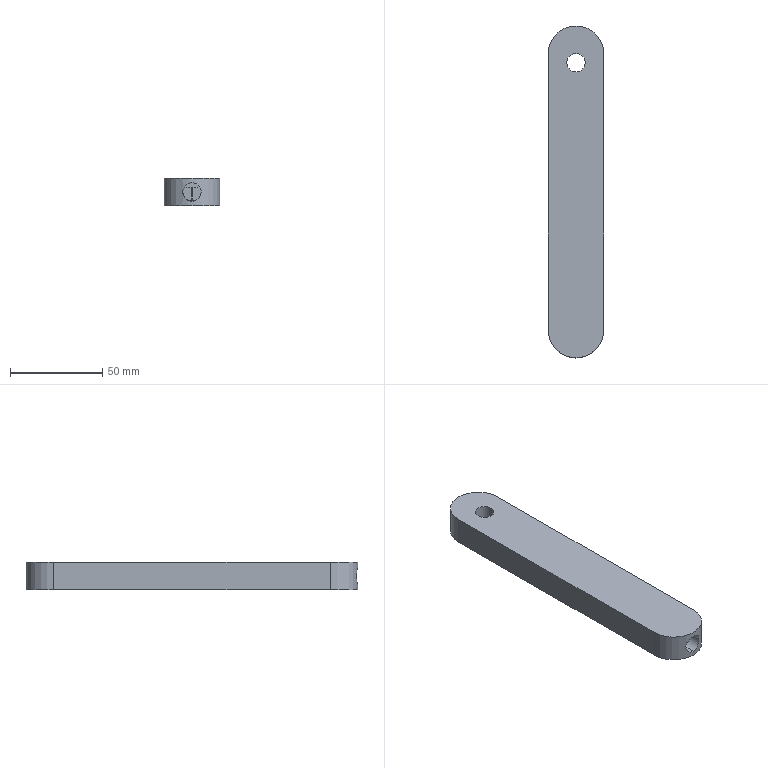Part | STEP file | 1 solid | 14 faces | box 30 x 180 x 15 mm | volume 74584 mm3 | cylinder 8 | plane 6 | commonest cylinder face diameters 10 x4 15 x2 30 x2